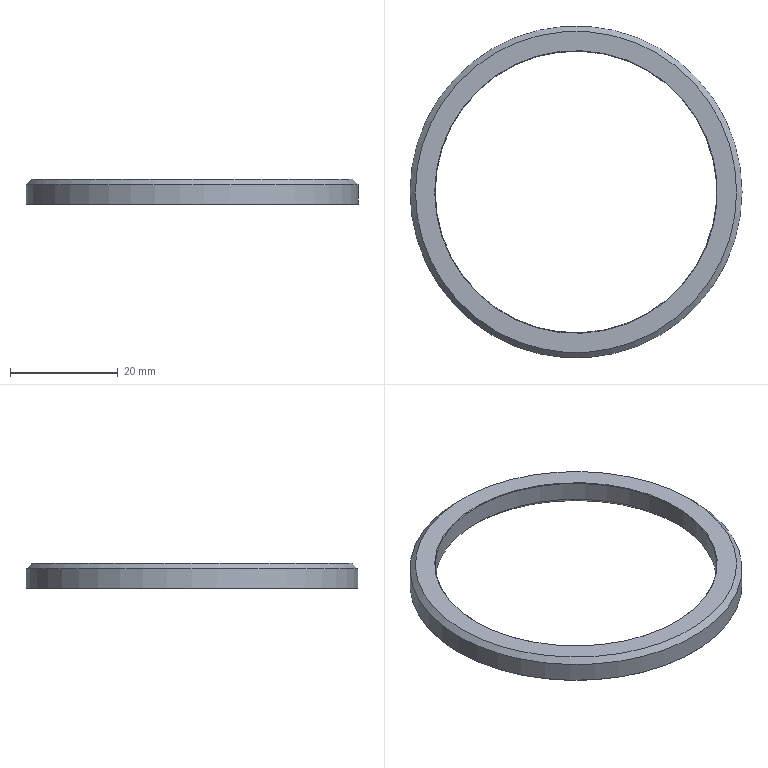Part | NX | features CHAMFER 4, DATUM_CSYS 2, EXTRUDE 1, SKETCH 1 | 1 solid | 8 faces | box 61.62 x 61.62 x 4.68 mm | volume 3737 mm3 | cone 4 | cylinder 2 | plane 2 | commonest cylinder face diameters 52.26 x1 61.62 x1
STEP:
#1=CARTESIAN_POINT('',(-30.81,0.,0.1));
#2=VERTEX_POINT('',#1);
#3=CARTESIAN_POINT('',(0.,0.,0.1));
#4=DIRECTION('',(0.,0.,-1.));
#5=DIRECTION('',(-1.,0.,0.));
#6=AXIS2_PLACEMENT_3D('',#3,#4,#5);
#7=CIRCLE('',#6,30.81);
#8=EDGE_CURVE('',#2,#2,#7,.F.);
#9=ORIENTED_EDGE('',*,*,#8,.T.);
#10=EDGE_LOOP('',(#9));
#11=FACE_BOUND('',#10,.T.);
#12=CARTESIAN_POINT('',(-30.81,0.,3.68));
#13=VERTEX_POINT('',#12);
#14=CARTESIAN_POINT('',(0.,0.,3.68));
#15=DIRECTION('',(0.,0.,-1.));
#16=DIRECTION('',(-1.,0.,0.));
#17=AXIS2_PLACEMENT_3D('',#14,#15,#16);
#18=CIRCLE('',#17,30.81);
#19=EDGE_CURVE('',#13,#13,#18,.T.);
#20=ORIENTED_EDGE('',*,*,#19,.T.);
#21=EDGE_LOOP('',(#20));
#22=FACE_BOUND('',#21,.T.);
#23=CARTESIAN_POINT('',(0.,0.,4.68));
#24=DIRECTION('',(0.,0.,-1.));
#25=DIRECTION('',(-1.,0.,0.));
#26=AXIS2_PLACEMENT_3D('',#23,#24,#25);
#27=CYLINDRICAL_SURFACE('',#26,30.81);
#28=ADVANCED_FACE('',(#11,#22),#27,.T.);
#29=CARTESIAN_POINT('',(-26.13,0.,1.));
#30=VERTEX_POINT('',#29);
#31=CARTESIAN_POINT('',(0.,0.,1.));
#32=DIRECTION('',(0.,0.,-1.));
#33=DIRECTION('',(-1.,0.,0.));
#34=AXIS2_PLACEMENT_3D('',#31,#32,#33);
#35=CIRCLE('',#34,26.13);
#36=EDGE_CURVE('',#30,#30,#35,.T.);
#37=ORIENTED_EDGE('',*,*,#36,.T.);
#38=EDGE_LOOP('',(#37));
#39=FACE_BOUND('',#38,.T.);
#40=CARTESIAN_POINT('',(-26.13,0.,4.58));
#41=VERTEX_POINT('',#40);
#42=CARTESIAN_POINT('',(0.,0.,4.58));
#43=DIRECTION('',(0.,0.,-1.));
#44=DIRECTION('',(-1.,0.,0.));
#45=AXIS2_PLACEMENT_3D('',#42,#43,#44);
#46=CIRCLE('',#45,26.13);
#47=EDGE_CURVE('',#41,#41,#46,.F.);
#48=ORIENTED_EDGE('',*,*,#47,.T.);
#49=EDGE_LOOP('',(#48));
#50=FACE_BOUND('',#49,.T.);
#51=CARTESIAN_POINT('',(0.,0.,4.68));
#52=DIRECTION('',(0.,0.,-1.));
#53=DIRECTION('',(-1.,0.,0.));
#54=AXIS2_PLACEMENT_3D('',#51,#52,#53);
#55=CYLINDRICAL_SURFACE('',#54,26.13);
#56=ADVANCED_FACE('',(#39,#50),#55,.F.);
#57=CARTESIAN_POINT('',(-26.23,0.,4.68));
#58=VERTEX_POINT('',#57);
#59=CARTESIAN_POINT('',(0.,0.,4.68));
#60=DIRECTION('',(0.,0.,-1.));
#61=DIRECTION('',(-1.,0.,0.));
#62=AXIS2_PLACEMENT_3D('',#59,#60,#61);
#63=CIRCLE('',#62,26.23);
#64=EDGE_CURVE('',#58,#58,#63,.T.);
#65=ORIENTED_EDGE('',*,*,#64,.T.);
#66=EDGE_LOOP('',(#65));
#67=FACE_BOUND('',#66,.T.);
#68=CARTESIAN_POINT('',(-29.81,0.,4.68));
#69=VERTEX_POINT('',#68);
#70=CARTESIAN_POINT('',(0.,0.,4.68));
#71=DIRECTION('',(0.,0.,-1.));
#72=DIRECTION('',(-1.,0.,0.));
#73=AXIS2_PLACEMENT_3D('',#70,#71,#72);
#74=CIRCLE('',#73,29.81);
#75=EDGE_CURVE('',#69,#69,#74,.F.);
#76=ORIENTED_EDGE('',*,*,#75,.T.);
#77=EDGE_LOOP('',(#76));
#78=FACE_BOUND('',#77,.T.);
#79=CARTESIAN_POINT('',(0.,0.,4.68));
#80=DIRECTION('',(0.,0.,-1.));
#81=DIRECTION('',(-1.,0.,0.));
#82=AXIS2_PLACEMENT_3D('',#79,#80,#81);
#83=PLANE('',#82);
#84=ADVANCED_FACE('',(#67,#78),#83,.F.);
#85=CARTESIAN_POINT('',(-27.13,0.,0.));
#86=VERTEX_POINT('',#85);
#87=CARTESIAN_POINT('',(0.,0.,0.));
#88=DIRECTION('',(0.,0.,-1.));
#89=DIRECTION('',(-1.,0.,0.));
#90=AXIS2_PLACEMENT_3D('',#87,#88,#89);
#91=CIRCLE('',#90,27.13);
#92=EDGE_CURVE('',#86,#86,#91,.F.);
#93=ORIENTED_EDGE('',*,*,#92,.T.);
#94=EDGE_LOOP('',(#93));
#95=FACE_BOUND('',#94,.T.);
#96=CARTESIAN_POINT('',(-30.71,0.,0.));
#97=VERTEX_POINT('',#96);
#98=CARTESIAN_POINT('',(0.,0.,0.));
#99=DIRECTION('',(0.,0.,-1.));
#100=DIRECTION('',(-1.,0.,0.));
#101=AXIS2_PLACEMENT_3D('',#98,#99,#100);
#102=CIRCLE('',#101,30.71);
#103=EDGE_CURVE('',#97,#97,#102,.T.);
#104=ORIENTED_EDGE('',*,*,#103,.T.);
#105=EDGE_LOOP('',(#104));
#106=FACE_BOUND('',#105,.T.);
#107=CARTESIAN_POINT('',(0.,0.,0.));
#108=DIRECTION('',(0.,0.,-1.));
#109=DIRECTION('',(-1.,0.,0.));
#110=AXIS2_PLACEMENT_3D('',#107,#108,#109);
#111=PLANE('',#110);
#112=ADVANCED_FACE('',(#95,#106),#111,.T.);
#113=ORIENTED_EDGE('',*,*,#75,.F.);
#114=EDGE_LOOP('',(#113));
#115=FACE_BOUND('',#114,.T.);
#116=ORIENTED_EDGE('',*,*,#19,.F.);
#117=EDGE_LOOP('',(#116));
#118=FACE_BOUND('',#117,.T.);
#119=CARTESIAN_POINT('',(0.,0.,3.68));
#120=DIRECTION('',(0.,0.,-1.));
#121=DIRECTION('',(-1.,0.,0.));
#122=AXIS2_PLACEMENT_3D('',#119,#120,#121);
#123=CONICAL_SURFACE('',#122,30.81,0.7854);
#124=ADVANCED_FACE('',(#115,#118),#123,.T.);
#125=ORIENTED_EDGE('',*,*,#8,.F.);
#126=EDGE_LOOP('',(#125));
#127=FACE_BOUND('',#126,.T.);
#128=ORIENTED_EDGE('',*,*,#103,.F.);
#129=EDGE_LOOP('',(#128));
#130=FACE_BOUND('',#129,.T.);
#131=CARTESIAN_POINT('',(0.,0.,0.));
#132=DIRECTION('',(0.,0.,1.));
#133=DIRECTION('',(1.,0.,0.));
#134=AXIS2_PLACEMENT_3D('',#131,#132,#133);
#135=CONICAL_SURFACE('',#134,30.71,0.7854);
#136=ADVANCED_FACE('',(#127,#130),#135,.T.);
#137=ORIENTED_EDGE('',*,*,#47,.F.);
#138=EDGE_LOOP('',(#137));
#139=FACE_BOUND('',#138,.T.);
#140=ORIENTED_EDGE('',*,*,#64,.F.);
#141=EDGE_LOOP('',(#140));
#142=FACE_BOUND('',#141,.T.);
#143=CARTESIAN_POINT('',(0.,0.,4.68));
#144=DIRECTION('',(0.,0.,1.));
#145=DIRECTION('',(1.,0.,0.));
#146=AXIS2_PLACEMENT_3D('',#143,#144,#145);
#147=CONICAL_SURFACE('',#146,26.23,0.7854);
#148=ADVANCED_FACE('',(#139,#142),#147,.F.);
#149=ORIENTED_EDGE('',*,*,#92,.F.);
#150=EDGE_LOOP('',(#149));
#151=FACE_BOUND('',#150,.T.);
#152=ORIENTED_EDGE('',*,*,#36,.F.);
#153=EDGE_LOOP('',(#152));
#154=FACE_BOUND('',#153,.T.);
#155=CARTESIAN_POINT('',(0.,0.,1.));
#156=DIRECTION('',(0.,0.,-1.));
#157=DIRECTION('',(-1.,0.,0.));
#158=AXIS2_PLACEMENT_3D('',#155,#156,#157);
#159=CONICAL_SURFACE('',#158,26.13,0.7854);
#160=ADVANCED_FACE('',(#151,#154),#159,.F.);
#161=CLOSED_SHELL('',(#28,#56,#84,#112,#124,#136,#148,#160));
#162=MANIFOLD_SOLID_BREP('',#161);
#163=(LENGTH_UNIT()NAMED_UNIT(*)SI_UNIT(.MILLI.,.METRE.));
#164=UNCERTAINTY_MEASURE_WITH_UNIT(LENGTH_MEASURE(0.00001),#163,'','');
#165=(NAMED_UNIT(*)PLANE_ANGLE_UNIT()SI_UNIT($,.RADIAN.));
#166=(NAMED_UNIT(*)SI_UNIT($,.STERADIAN.)SOLID_ANGLE_UNIT());
#167=(GEOMETRIC_REPRESENTATION_CONTEXT(3)GLOBAL_UNCERTAINTY_ASSIGNED_CONTEXT((#164))GLOBAL_UNIT_ASSIGNED_CONTEXT((#163,#165,#166))REPRESENTATION_CONTEXT('',''));
#168=ADVANCED_BREP_SHAPE_REPRESENTATION('',(#162),#167);